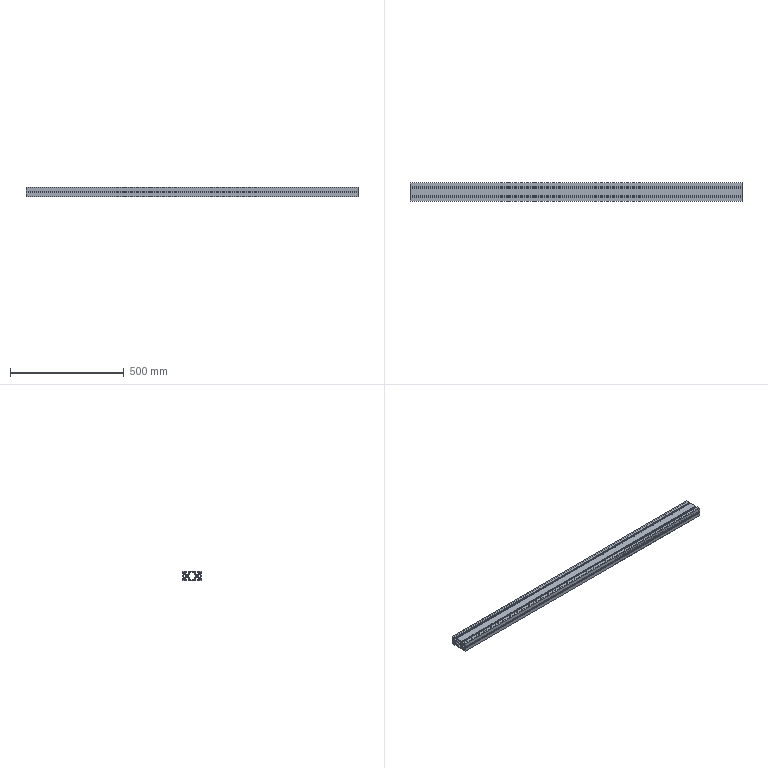Part | SolidWorks | features BaseBody 1 | 1 solid | 90 faces | box 1460 x 80 x 40 mm | volume 1799358 mm3 | plane 66 | cylinder 24 | commonest cylinder face diameters 10 x12 8 x8 6.2 x4